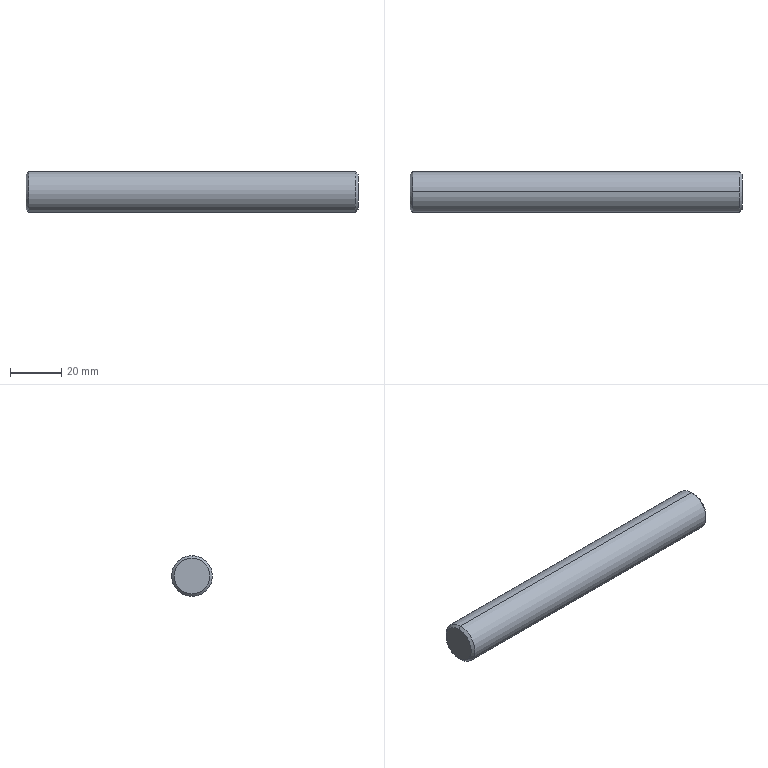Part | STEP file | BB67-M16-130L | 1 solid | 8 faces | box 130 x 16 x 16 mm | volume 26090 mm3 | cone 4 | cylinder 2 | plane 2 | commonest cylinder face diameters 16 x2
STEP:
#1=CARTESIAN_POINT('',(150.,10.,-7.));
#2=VERTEX_POINT('',#1);
#3=CARTESIAN_POINT('',(150.,10.,7.));
#4=VERTEX_POINT('',#3);
#5=CARTESIAN_POINT('',(150.,10.,0.));
#6=DIRECTION('',(1.,0.,0.));
#7=DIRECTION('',(0.,0.,-1.));
#8=AXIS2_PLACEMENT_3D('',#5,#6,#7);
#9=CIRCLE('',#8,7.);
#10=EDGE_CURVE('',#2,#4,#9,.T.);
#11=ORIENTED_EDGE('',*,*,#10,.F.);
#12=CARTESIAN_POINT('',(149.,10.,-8.));
#13=VERTEX_POINT('',#12);
#14=CARTESIAN_POINT('',(149.,10.,-8.));
#15=DIRECTION('',(-0.7071,0.,-0.7071));
#16=VECTOR('',#15,1000.);
#17=LINE('',#14,#16);
#18=EDGE_CURVE('',#2,#13,#17,.T.);
#19=ORIENTED_EDGE('',*,*,#18,.T.);
#20=CARTESIAN_POINT('',(149.,10.,8.));
#21=VERTEX_POINT('',#20);
#22=CARTESIAN_POINT('',(149.,10.,0.));
#23=DIRECTION('',(-1.,0.,0.));
#24=DIRECTION('',(0.,0.,-1.));
#25=AXIS2_PLACEMENT_3D('',#22,#23,#24);
#26=CIRCLE('',#25,8.);
#27=EDGE_CURVE('',#21,#13,#26,.T.);
#28=ORIENTED_EDGE('',*,*,#27,.F.);
#29=CARTESIAN_POINT('',(149.,10.,8.));
#30=DIRECTION('',(-0.7071,0.,0.7071));
#31=VECTOR('',#30,1000.);
#32=LINE('',#29,#31);
#33=EDGE_CURVE('',#4,#21,#32,.T.);
#34=ORIENTED_EDGE('',*,*,#33,.F.);
#35=EDGE_LOOP('',(#11,#19,#28,#34));
#36=FACE_OUTER_BOUND('',#35,.T.);
#37=CARTESIAN_POINT('',(149.,10.,0.));
#38=DIRECTION('',(-1.,0.,0.));
#39=DIRECTION('',(0.,0.,1.));
#40=AXIS2_PLACEMENT_3D('',#37,#38,#39);
#41=CONICAL_SURFACE('',#40,8.,0.7854);
#42=ADVANCED_FACE('',(#36),#41,.T.);
#43=CARTESIAN_POINT('',(20.,10.,7.));
#44=VERTEX_POINT('',#43);
#45=CARTESIAN_POINT('',(20.,10.,-7.));
#46=VERTEX_POINT('',#45);
#47=CARTESIAN_POINT('',(20.,10.,0.));
#48=DIRECTION('',(-1.,0.,0.));
#49=DIRECTION('',(0.,0.,1.));
#50=AXIS2_PLACEMENT_3D('',#47,#48,#49);
#51=CIRCLE('',#50,7.);
#52=EDGE_CURVE('',#44,#46,#51,.T.);
#53=ORIENTED_EDGE('',*,*,#52,.F.);
#54=CARTESIAN_POINT('',(21.,10.,8.));
#55=VERTEX_POINT('',#54);
#56=CARTESIAN_POINT('',(21.,10.,8.));
#57=DIRECTION('',(0.7071,0.,0.7071));
#58=VECTOR('',#57,1000.);
#59=LINE('',#56,#58);
#60=EDGE_CURVE('',#44,#55,#59,.T.);
#61=ORIENTED_EDGE('',*,*,#60,.T.);
#62=CARTESIAN_POINT('',(21.,10.,-8.));
#63=VERTEX_POINT('',#62);
#64=CARTESIAN_POINT('',(21.,10.,0.));
#65=DIRECTION('',(1.,0.,0.));
#66=DIRECTION('',(0.,0.,1.));
#67=AXIS2_PLACEMENT_3D('',#64,#65,#66);
#68=CIRCLE('',#67,8.);
#69=EDGE_CURVE('',#63,#55,#68,.T.);
#70=ORIENTED_EDGE('',*,*,#69,.F.);
#71=CARTESIAN_POINT('',(21.,10.,-8.));
#72=DIRECTION('',(0.7071,0.,-0.7071));
#73=VECTOR('',#72,1000.);
#74=LINE('',#71,#73);
#75=EDGE_CURVE('',#46,#63,#74,.T.);
#76=ORIENTED_EDGE('',*,*,#75,.F.);
#77=EDGE_LOOP('',(#53,#61,#70,#76));
#78=FACE_OUTER_BOUND('',#77,.T.);
#79=CARTESIAN_POINT('',(21.,10.,0.));
#80=DIRECTION('',(1.,0.,0.));
#81=DIRECTION('',(0.,0.,-1.));
#82=AXIS2_PLACEMENT_3D('',#79,#80,#81);
#83=CONICAL_SURFACE('',#82,8.,0.7854);
#84=ADVANCED_FACE('',(#78),#83,.T.);
#85=ORIENTED_EDGE('',*,*,#69,.T.);
#86=CARTESIAN_POINT('',(20.,10.,8.));
#87=DIRECTION('',(1.,0.,0.));
#88=VECTOR('',#87,1000.);
#89=LINE('',#86,#88);
#90=EDGE_CURVE('',#55,#21,#89,.T.);
#91=ORIENTED_EDGE('',*,*,#90,.T.);
#92=ORIENTED_EDGE('',*,*,#27,.T.);
#93=CARTESIAN_POINT('',(20.,10.,-8.));
#94=DIRECTION('',(1.,0.,0.));
#95=VECTOR('',#94,1000.);
#96=LINE('',#93,#95);
#97=EDGE_CURVE('',#63,#13,#96,.T.);
#98=ORIENTED_EDGE('',*,*,#97,.F.);
#99=EDGE_LOOP('',(#85,#91,#92,#98));
#100=FACE_OUTER_BOUND('',#99,.T.);
#101=CARTESIAN_POINT('',(20.,10.,0.));
#102=DIRECTION('',(1.,0.,0.));
#103=DIRECTION('',(0.,0.,-1.));
#104=AXIS2_PLACEMENT_3D('',#101,#102,#103);
#105=CYLINDRICAL_SURFACE('',#104,8.);
#106=ADVANCED_FACE('',(#100),#105,.T.);
#107=CARTESIAN_POINT('',(150.,10.,0.));
#108=DIRECTION('',(1.,0.,0.));
#109=DIRECTION('',(0.,0.,-1.));
#110=AXIS2_PLACEMENT_3D('',#107,#108,#109);
#111=CIRCLE('',#110,7.);
#112=EDGE_CURVE('',#4,#2,#111,.T.);
#113=ORIENTED_EDGE('',*,*,#112,.T.);
#114=ORIENTED_EDGE('',*,*,#10,.T.);
#115=EDGE_LOOP('',(#113,#114));
#116=FACE_OUTER_BOUND('',#115,.T.);
#117=CARTESIAN_POINT('',(150.,10.,0.));
#118=DIRECTION('',(1.,0.,0.));
#119=DIRECTION('',(0.,0.,-1.));
#120=AXIS2_PLACEMENT_3D('',#117,#118,#119);
#121=PLANE('',#120);
#122=ADVANCED_FACE('',(#116),#121,.T.);
#123=CARTESIAN_POINT('',(20.,10.,0.));
#124=DIRECTION('',(-1.,0.,0.));
#125=DIRECTION('',(0.,0.,1.));
#126=AXIS2_PLACEMENT_3D('',#123,#124,#125);
#127=CIRCLE('',#126,7.);
#128=EDGE_CURVE('',#46,#44,#127,.T.);
#129=ORIENTED_EDGE('',*,*,#128,.T.);
#130=ORIENTED_EDGE('',*,*,#52,.T.);
#131=EDGE_LOOP('',(#129,#130));
#132=FACE_OUTER_BOUND('',#131,.T.);
#133=CARTESIAN_POINT('',(20.,10.,0.));
#134=DIRECTION('',(-1.,0.,0.));
#135=DIRECTION('',(0.,0.,1.));
#136=AXIS2_PLACEMENT_3D('',#133,#134,#135);
#137=PLANE('',#136);
#138=ADVANCED_FACE('',(#132),#137,.T.);
#139=ORIENTED_EDGE('',*,*,#90,.F.);
#140=CARTESIAN_POINT('',(21.,10.,0.));
#141=DIRECTION('',(1.,0.,0.));
#142=DIRECTION('',(0.,0.,1.));
#143=AXIS2_PLACEMENT_3D('',#140,#141,#142);
#144=CIRCLE('',#143,8.);
#145=EDGE_CURVE('',#55,#63,#144,.T.);
#146=ORIENTED_EDGE('',*,*,#145,.T.);
#147=ORIENTED_EDGE('',*,*,#97,.T.);
#148=CARTESIAN_POINT('',(149.,10.,0.));
#149=DIRECTION('',(-1.,0.,0.));
#150=DIRECTION('',(0.,0.,-1.));
#151=AXIS2_PLACEMENT_3D('',#148,#149,#150);
#152=CIRCLE('',#151,8.);
#153=EDGE_CURVE('',#13,#21,#152,.T.);
#154=ORIENTED_EDGE('',*,*,#153,.T.);
#155=EDGE_LOOP('',(#139,#146,#147,#154));
#156=FACE_OUTER_BOUND('',#155,.T.);
#157=CARTESIAN_POINT('',(20.,10.,0.));
#158=DIRECTION('',(1.,0.,0.));
#159=DIRECTION('',(0.,0.,-1.));
#160=AXIS2_PLACEMENT_3D('',#157,#158,#159);
#161=CYLINDRICAL_SURFACE('',#160,8.);
#162=ADVANCED_FACE('',(#156),#161,.T.);
#163=ORIENTED_EDGE('',*,*,#60,.F.);
#164=ORIENTED_EDGE('',*,*,#128,.F.);
#165=ORIENTED_EDGE('',*,*,#75,.T.);
#166=ORIENTED_EDGE('',*,*,#145,.F.);
#167=EDGE_LOOP('',(#163,#164,#165,#166));
#168=FACE_OUTER_BOUND('',#167,.T.);
#169=CARTESIAN_POINT('',(21.,10.,0.));
#170=DIRECTION('',(1.,0.,0.));
#171=DIRECTION('',(0.,0.,-1.));
#172=AXIS2_PLACEMENT_3D('',#169,#170,#171);
#173=CONICAL_SURFACE('',#172,8.,0.7854);
#174=ADVANCED_FACE('',(#168),#173,.T.);
#175=ORIENTED_EDGE('',*,*,#18,.F.);
#176=ORIENTED_EDGE('',*,*,#112,.F.);
#177=ORIENTED_EDGE('',*,*,#33,.T.);
#178=ORIENTED_EDGE('',*,*,#153,.F.);
#179=EDGE_LOOP('',(#175,#176,#177,#178));
#180=FACE_OUTER_BOUND('',#179,.T.);
#181=CARTESIAN_POINT('',(149.,10.,0.));
#182=DIRECTION('',(-1.,0.,0.));
#183=DIRECTION('',(0.,0.,1.));
#184=AXIS2_PLACEMENT_3D('',#181,#182,#183);
#185=CONICAL_SURFACE('',#184,8.,0.7854);
#186=ADVANCED_FACE('',(#180),#185,.T.);
#187=CLOSED_SHELL('',(#42,#84,#106,#122,#138,#162,#174,#186));
#188=MANIFOLD_SOLID_BREP('',#187);
#189=CARTESIAN_POINT('',(0.,0.,0.));
#190=DIRECTION('',(0.,0.,1.));
#191=DIRECTION('',(1.,0.,0.));
#192=AXIS2_PLACEMENT_3D('',#189,#190,#191);
#193=(LENGTH_UNIT()NAMED_UNIT(*)SI_UNIT(.MILLI.,.METRE.));
#194=UNCERTAINTY_MEASURE_WITH_UNIT(LENGTH_MEASURE(0.00001),#193,'','');
#195=(NAMED_UNIT(*)PLANE_ANGLE_UNIT()SI_UNIT($,.RADIAN.));
#196=(NAMED_UNIT(*)SI_UNIT($,.STERADIAN.)SOLID_ANGLE_UNIT());
#197=(GEOMETRIC_REPRESENTATION_CONTEXT(3)GLOBAL_UNCERTAINTY_ASSIGNED_CONTEXT((#194))GLOBAL_UNIT_ASSIGNED_CONTEXT((#193,#195,#196))REPRESENTATION_CONTEXT('',''));
#198=ADVANCED_BREP_SHAPE_REPRESENTATION('',(#188,#192),#197);